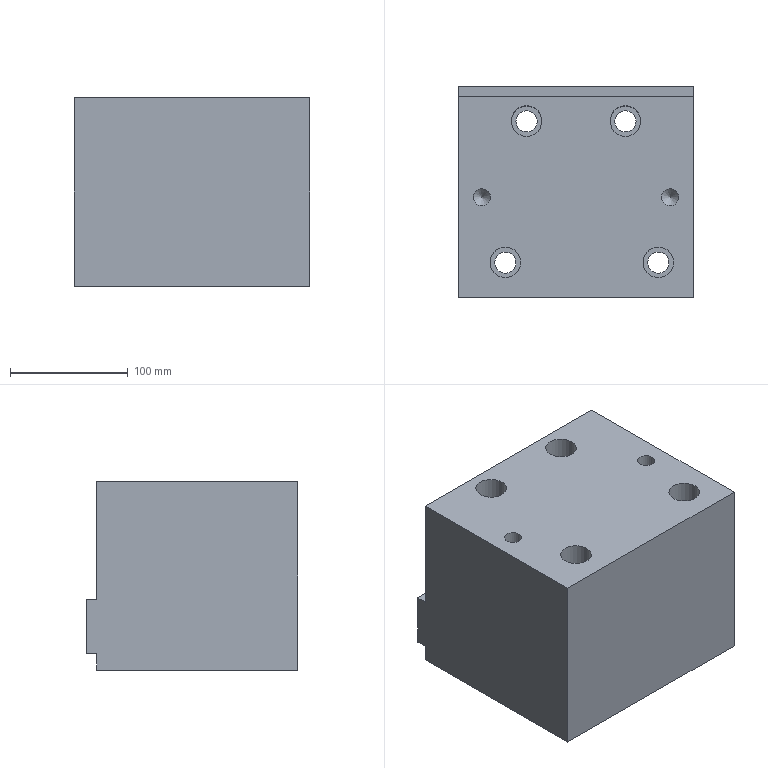Part | STEP file | lll_id4218_x_t | 1 solid | 34 faces | box 200 x 180 x 160 mm | volume 5239112 mm3 | plane 14 | cylinder 14 | cone 6 | commonest cylinder face diameters 8.506 x4 18.009 x4 26.008 x4 14.506 x2
STEP:
#1=CARTESIAN_POINT('',(1841.005,-387.377,-55.));
#2=VERTEX_POINT('',#1);
#3=CARTESIAN_POINT('',(1832.,-387.377,-55.));
#4=DIRECTION('',(0.,0.,1.));
#5=DIRECTION('',(1.,0.,0.));
#6=AXIS2_PLACEMENT_3D('',#3,#4,#5);
#7=CIRCLE('',#6,9.005);
#8=EDGE_CURVE('',#2,#2,#7,.T.);
#9=ORIENTED_EDGE('',*,*,#8,.F.);
#10=EDGE_LOOP('',(#9));
#11=FACE_BOUND('',#10,.T.);
#12=CARTESIAN_POINT('',(1845.004,-387.377,-55.));
#13=VERTEX_POINT('',#12);
#14=CARTESIAN_POINT('',(1832.,-387.377,-55.));
#15=DIRECTION('',(0.,0.,1.));
#16=DIRECTION('',(1.,0.,0.));
#17=AXIS2_PLACEMENT_3D('',#14,#15,#16);
#18=CIRCLE('',#17,13.004);
#19=EDGE_CURVE('',#13,#13,#18,.T.);
#20=ORIENTED_EDGE('',*,*,#19,.T.);
#21=EDGE_LOOP('',(#20));
#22=FACE_BOUND('',#21,.T.);
#23=CARTESIAN_POINT('',(1832.,-387.377,-55.));
#24=DIRECTION('',(0.,0.,-1.));
#25=DIRECTION('',(-1.,0.,0.));
#26=AXIS2_PLACEMENT_3D('',#23,#24,#25);
#27=PLANE('',#26);
#28=ADVANCED_FACE('',(#11,#22),#27,.F.);
#29=ORIENTED_EDGE('',*,*,#8,.T.);
#30=EDGE_LOOP('',(#29));
#31=FACE_BOUND('',#30,.T.);
#32=CARTESIAN_POINT('',(1841.005,-387.377,-95.));
#33=VERTEX_POINT('',#32);
#34=CARTESIAN_POINT('',(1832.,-387.377,-95.));
#35=DIRECTION('',(0.,0.,1.));
#36=DIRECTION('',(1.,0.,0.));
#37=AXIS2_PLACEMENT_3D('',#34,#35,#36);
#38=CIRCLE('',#37,9.005);
#39=EDGE_CURVE('',#33,#33,#38,.T.);
#40=ORIENTED_EDGE('',*,*,#39,.F.);
#41=EDGE_LOOP('',(#40));
#42=FACE_BOUND('',#41,.T.);
#43=CARTESIAN_POINT('',(1832.,-387.377,67.));
#44=DIRECTION('',(0.,0.,-1.));
#45=DIRECTION('',(1.,0.,0.));
#46=AXIS2_PLACEMENT_3D('',#43,#44,#45);
#47=CYLINDRICAL_SURFACE('',#46,9.005);
#48=ADVANCED_FACE('',(#31,#42),#47,.F.);
#49=ORIENTED_EDGE('',*,*,#19,.F.);
#50=EDGE_LOOP('',(#49));
#51=FACE_BOUND('',#50,.T.);
#52=CARTESIAN_POINT('',(1845.004,-387.377,65.));
#53=VERTEX_POINT('',#52);
#54=CARTESIAN_POINT('',(1832.,-387.377,65.));
#55=DIRECTION('',(0.,0.,1.));
#56=DIRECTION('',(1.,0.,0.));
#57=AXIS2_PLACEMENT_3D('',#54,#55,#56);
#58=CIRCLE('',#57,13.004);
#59=EDGE_CURVE('',#53,#53,#58,.T.);
#60=ORIENTED_EDGE('',*,*,#59,.T.);
#61=EDGE_LOOP('',(#60));
#62=FACE_BOUND('',#61,.T.);
#63=CARTESIAN_POINT('',(1832.,-387.377,65.));
#64=DIRECTION('',(0.,0.,-1.));
#65=DIRECTION('',(1.,0.,0.));
#66=AXIS2_PLACEMENT_3D('',#63,#64,#65);
#67=CYLINDRICAL_SURFACE('',#66,13.004);
#68=ADVANCED_FACE('',(#51,#62),#67,.F.);
#69=CARTESIAN_POINT('',(1715.,-401.383,40.));
#70=VERTEX_POINT('',#69);
#71=VERTEX_LOOP('',#70);
#72=FACE_BOUND('',#71,.T.);
#73=CARTESIAN_POINT('',(1715.,-397.13,35.747));
#74=VERTEX_POINT('',#73);
#75=CARTESIAN_POINT('',(1715.,-397.13,40.));
#76=DIRECTION('',(0.,1.,0.));
#77=DIRECTION('',(0.,0.,-1.));
#78=AXIS2_PLACEMENT_3D('',#75,#76,#77);
#79=CIRCLE('',#78,4.253);
#80=EDGE_CURVE('',#74,#74,#79,.T.);
#81=ORIENTED_EDGE('',*,*,#80,.T.);
#82=EDGE_LOOP('',(#81));
#83=FACE_BOUND('',#82,.T.);
#84=CARTESIAN_POINT('',(1715.,-397.13,40.));
#85=DIRECTION('',(0.,1.,0.));
#86=DIRECTION('',(0.,0.,1.));
#87=AXIS2_PLACEMENT_3D('',#84,#85,#86);
#88=CONICAL_SURFACE('',#87,4.253,45.);
#89=ADVANCED_FACE('',(#72,#83),#88,.F.);
#90=CARTESIAN_POINT('',(1865.,-401.383,40.));
#91=VERTEX_POINT('',#90);
#92=VERTEX_LOOP('',#91);
#93=FACE_BOUND('',#92,.T.);
#94=CARTESIAN_POINT('',(1865.,-397.13,35.747));
#95=VERTEX_POINT('',#94);
#96=CARTESIAN_POINT('',(1865.,-397.13,40.));
#97=DIRECTION('',(0.,1.,0.));
#98=DIRECTION('',(0.,0.,-1.));
#99=AXIS2_PLACEMENT_3D('',#96,#97,#98);
#100=CIRCLE('',#99,4.253);
#101=EDGE_CURVE('',#95,#95,#100,.T.);
#102=ORIENTED_EDGE('',*,*,#101,.T.);
#103=EDGE_LOOP('',(#102));
#104=FACE_BOUND('',#103,.T.);
#105=CARTESIAN_POINT('',(1865.,-397.13,40.));
#106=DIRECTION('',(0.,1.,0.));
#107=DIRECTION('',(0.,0.,1.));
#108=AXIS2_PLACEMENT_3D('',#105,#106,#107);
#109=CONICAL_SURFACE('',#108,4.253,45.);
#110=ADVANCED_FACE('',(#93,#104),#109,.F.);
#111=CARTESIAN_POINT('',(1715.,-401.383,-10.));
#112=VERTEX_POINT('',#111);
#113=VERTEX_LOOP('',#112);
#114=FACE_BOUND('',#113,.T.);
#115=CARTESIAN_POINT('',(1715.,-397.13,-14.253));
#116=VERTEX_POINT('',#115);
#117=CARTESIAN_POINT('',(1715.,-397.13,-10.));
#118=DIRECTION('',(0.,1.,0.));
#119=DIRECTION('',(0.,0.,-1.));
#120=AXIS2_PLACEMENT_3D('',#117,#118,#119);
#121=CIRCLE('',#120,4.253);
#122=EDGE_CURVE('',#116,#116,#121,.T.);
#123=ORIENTED_EDGE('',*,*,#122,.T.);
#124=EDGE_LOOP('',(#123));
#125=FACE_BOUND('',#124,.T.);
#126=CARTESIAN_POINT('',(1715.,-397.13,-10.));
#127=DIRECTION('',(0.,1.,0.));
#128=DIRECTION('',(0.,0.,1.));
#129=AXIS2_PLACEMENT_3D('',#126,#127,#128);
#130=CONICAL_SURFACE('',#129,4.253,45.);
#131=ADVANCED_FACE('',(#114,#125),#130,.F.);
#132=CARTESIAN_POINT('',(1865.,-401.383,-10.));
#133=VERTEX_POINT('',#132);
#134=VERTEX_LOOP('',#133);
#135=FACE_BOUND('',#134,.T.);
#136=CARTESIAN_POINT('',(1865.,-397.13,-14.253));
#137=VERTEX_POINT('',#136);
#138=CARTESIAN_POINT('',(1865.,-397.13,-10.));
#139=DIRECTION('',(0.,1.,0.));
#140=DIRECTION('',(0.,0.,-1.));
#141=AXIS2_PLACEMENT_3D('',#138,#139,#140);
#142=CIRCLE('',#141,4.253);
#143=EDGE_CURVE('',#137,#137,#142,.T.);
#144=ORIENTED_EDGE('',*,*,#143,.T.);
#145=EDGE_LOOP('',(#144));
#146=FACE_BOUND('',#145,.T.);
#147=CARTESIAN_POINT('',(1865.,-397.13,-10.));
#148=DIRECTION('',(0.,1.,0.));
#149=DIRECTION('',(0.,0.,1.));
#150=AXIS2_PLACEMENT_3D('',#147,#148,#149);
#151=CONICAL_SURFACE('',#150,4.253,45.);
#152=ADVANCED_FACE('',(#135,#146),#151,.F.);
#153=CARTESIAN_POINT('',(1710.,-451.877,21.994));
#154=VERTEX_POINT('',#153);
#155=VERTEX_LOOP('',#154);
#156=FACE_BOUND('',#155,.T.);
#157=CARTESIAN_POINT('',(1717.253,-451.877,29.247));
#158=VERTEX_POINT('',#157);
#159=CARTESIAN_POINT('',(1710.,-451.877,29.247));
#160=DIRECTION('',(0.,0.,1.));
#161=DIRECTION('',(1.,0.,0.));
#162=AXIS2_PLACEMENT_3D('',#159,#160,#161);
#163=CIRCLE('',#162,7.253);
#164=EDGE_CURVE('',#158,#158,#163,.T.);
#165=ORIENTED_EDGE('',*,*,#164,.T.);
#166=EDGE_LOOP('',(#165));
#167=FACE_BOUND('',#166,.T.);
#168=CARTESIAN_POINT('',(1710.,-451.877,29.247));
#169=DIRECTION('',(0.,0.,1.));
#170=DIRECTION('',(-1.,0.,0.));
#171=AXIS2_PLACEMENT_3D('',#168,#169,#170);
#172=CONICAL_SURFACE('',#171,7.253,45.);
#173=ADVANCED_FACE('',(#156,#167),#172,.F.);
#174=ORIENTED_EDGE('',*,*,#80,.F.);
#175=EDGE_LOOP('',(#174));
#176=FACE_BOUND('',#175,.T.);
#177=CARTESIAN_POINT('',(1710.747,-366.377,40.));
#178=VERTEX_POINT('',#177);
#179=CARTESIAN_POINT('',(1715.,-366.377,40.));
#180=DIRECTION('',(0.,1.,0.));
#181=DIRECTION('',(-1.,0.,0.));
#182=AXIS2_PLACEMENT_3D('',#179,#180,#181);
#183=CIRCLE('',#182,4.253);
#184=EDGE_CURVE('',#178,#178,#183,.T.);
#185=ORIENTED_EDGE('',*,*,#184,.T.);
#186=EDGE_LOOP('',(#185));
#187=FACE_BOUND('',#186,.T.);
#188=CARTESIAN_POINT('',(1715.,-366.377,40.));
#189=DIRECTION('',(0.,-1.,0.));
#190=DIRECTION('',(-1.,0.,0.));
#191=AXIS2_PLACEMENT_3D('',#188,#189,#190);
#192=CYLINDRICAL_SURFACE('',#191,4.253);
#193=ADVANCED_FACE('',(#176,#187),#192,.F.);
#194=ORIENTED_EDGE('',*,*,#101,.F.);
#195=EDGE_LOOP('',(#194));
#196=FACE_BOUND('',#195,.T.);
#197=CARTESIAN_POINT('',(1860.747,-366.377,40.));
#198=VERTEX_POINT('',#197);
#199=CARTESIAN_POINT('',(1865.,-366.377,40.));
#200=DIRECTION('',(0.,1.,0.));
#201=DIRECTION('',(-1.,0.,0.));
#202=AXIS2_PLACEMENT_3D('',#199,#200,#201);
#203=CIRCLE('',#202,4.253);
#204=EDGE_CURVE('',#198,#198,#203,.T.);
#205=ORIENTED_EDGE('',*,*,#204,.T.);
#206=EDGE_LOOP('',(#205));
#207=FACE_BOUND('',#206,.T.);
#208=CARTESIAN_POINT('',(1865.,-366.377,40.));
#209=DIRECTION('',(0.,-1.,0.));
#210=DIRECTION('',(-1.,0.,0.));
#211=AXIS2_PLACEMENT_3D('',#208,#209,#210);
#212=CYLINDRICAL_SURFACE('',#211,4.253);
#213=ADVANCED_FACE('',(#196,#207),#212,.F.);
#214=ORIENTED_EDGE('',*,*,#122,.F.);
#215=EDGE_LOOP('',(#214));
#216=FACE_BOUND('',#215,.T.);
#217=CARTESIAN_POINT('',(1710.747,-366.377,-10.));
#218=VERTEX_POINT('',#217);
#219=CARTESIAN_POINT('',(1715.,-366.377,-10.));
#220=DIRECTION('',(0.,1.,0.));
#221=DIRECTION('',(-1.,0.,0.));
#222=AXIS2_PLACEMENT_3D('',#219,#220,#221);
#223=CIRCLE('',#222,4.253);
#224=EDGE_CURVE('',#218,#218,#223,.T.);
#225=ORIENTED_EDGE('',*,*,#224,.T.);
#226=EDGE_LOOP('',(#225));
#227=FACE_BOUND('',#226,.T.);
#228=CARTESIAN_POINT('',(1715.,-366.377,-10.));
#229=DIRECTION('',(0.,-1.,0.));
#230=DIRECTION('',(-1.,0.,0.));
#231=AXIS2_PLACEMENT_3D('',#228,#229,#230);
#232=CYLINDRICAL_SURFACE('',#231,4.253);
#233=ADVANCED_FACE('',(#216,#227),#232,.F.);
#234=ORIENTED_EDGE('',*,*,#143,.F.);
#235=EDGE_LOOP('',(#234));
#236=FACE_BOUND('',#235,.T.);
#237=CARTESIAN_POINT('',(1860.747,-366.377,-10.));
#238=VERTEX_POINT('',#237);
#239=CARTESIAN_POINT('',(1865.,-366.377,-10.));
#240=DIRECTION('',(0.,1.,0.));
#241=DIRECTION('',(-1.,0.,0.));
#242=AXIS2_PLACEMENT_3D('',#239,#240,#241);
#243=CIRCLE('',#242,4.253);
#244=EDGE_CURVE('',#238,#238,#243,.T.);
#245=ORIENTED_EDGE('',*,*,#244,.T.);
#246=EDGE_LOOP('',(#245));
#247=FACE_BOUND('',#246,.T.);
#248=CARTESIAN_POINT('',(1865.,-366.377,-10.));
#249=DIRECTION('',(0.,-1.,0.));
#250=DIRECTION('',(-1.,0.,0.));
#251=AXIS2_PLACEMENT_3D('',#248,#249,#250);
#252=CYLINDRICAL_SURFACE('',#251,4.253);
#253=ADVANCED_FACE('',(#236,#247),#252,.F.);
#254=CARTESIAN_POINT('',(1738.995,-387.377,-55.));
#255=VERTEX_POINT('',#254);
#256=CARTESIAN_POINT('',(1748.,-387.377,-55.));
#257=DIRECTION('',(0.,0.,1.));
#258=DIRECTION('',(-1.,0.,0.));
#259=AXIS2_PLACEMENT_3D('',#256,#257,#258);
#260=CIRCLE('',#259,9.005);
#261=EDGE_CURVE('',#255,#255,#260,.T.);
#262=ORIENTED_EDGE('',*,*,#261,.F.);
#263=EDGE_LOOP('',(#262));
#264=FACE_BOUND('',#263,.T.);
#265=CARTESIAN_POINT('',(1734.996,-387.377,-55.));
#266=VERTEX_POINT('',#265);
#267=CARTESIAN_POINT('',(1748.,-387.377,-55.));
#268=DIRECTION('',(0.,0.,1.));
#269=DIRECTION('',(-1.,0.,0.));
#270=AXIS2_PLACEMENT_3D('',#267,#268,#269);
#271=CIRCLE('',#270,13.004);
#272=EDGE_CURVE('',#266,#266,#271,.T.);
#273=ORIENTED_EDGE('',*,*,#272,.T.);
#274=EDGE_LOOP('',(#273));
#275=FACE_BOUND('',#274,.T.);
#276=CARTESIAN_POINT('',(1748.,-387.377,-55.));
#277=DIRECTION('',(0.,0.,-1.));
#278=DIRECTION('',(1.,0.,0.));
#279=AXIS2_PLACEMENT_3D('',#276,#277,#278);
#280=PLANE('',#279);
#281=ADVANCED_FACE('',(#264,#275),#280,.F.);
#282=CARTESIAN_POINT('',(1690.,-366.377,-35.));
#283=VERTEX_POINT('',#282);
#284=CARTESIAN_POINT('',(1890.,-366.377,-35.));
#285=VERTEX_POINT('',#284);
#286=CARTESIAN_POINT('',(1142.435,-366.377,-35.));
#287=DIRECTION('',(1.,0.,0.));
#288=VECTOR('',#287,1.);
#289=LINE('',#286,#288);
#290=EDGE_CURVE('',#283,#285,#289,.T.);
#291=ORIENTED_EDGE('',*,*,#290,.T.);
#292=CARTESIAN_POINT('',(1890.,-357.377,-35.));
#293=VERTEX_POINT('',#292);
#294=CARTESIAN_POINT('',(1890.,-26.33,-35.));
#295=DIRECTION('',(0.,-1.,0.));
#296=VECTOR('',#295,1.);
#297=LINE('',#294,#296);
#298=EDGE_CURVE('',#293,#285,#297,.T.);
#299=ORIENTED_EDGE('',*,*,#298,.F.);
#300=CARTESIAN_POINT('',(1690.,-357.377,-35.));
#301=VERTEX_POINT('',#300);
#302=CARTESIAN_POINT('',(1142.435,-357.377,-35.));
#303=DIRECTION('',(-1.,0.,0.));
#304=VECTOR('',#303,1.);
#305=LINE('',#302,#304);
#306=EDGE_CURVE('',#293,#301,#305,.T.);
#307=ORIENTED_EDGE('',*,*,#306,.T.);
#308=CARTESIAN_POINT('',(1690.,-376.377,-35.));
#309=DIRECTION('',(0.,-1.,0.));
#310=VECTOR('',#309,1.);
#311=LINE('',#308,#310);
#312=EDGE_CURVE('',#301,#283,#311,.T.);
#313=ORIENTED_EDGE('',*,*,#312,.T.);
#314=EDGE_LOOP('',(#291,#299,#307,#313));
#315=FACE_OUTER_BOUND('',#314,.T.);
#316=CARTESIAN_POINT('',(1142.435,-26.33,-35.));
#317=DIRECTION('',(0.,0.,1.));
#318=DIRECTION('',(1.,0.,0.));
#319=AXIS2_PLACEMENT_3D('',#316,#317,#318);
#320=PLANE('',#319);
#321=ADVANCED_FACE('',(#315),#320,.T.);
#322=CARTESIAN_POINT('',(1720.995,-507.377,-55.));
#323=VERTEX_POINT('',#322);
#324=CARTESIAN_POINT('',(1730.,-507.377,-55.));
#325=DIRECTION('',(0.,0.,1.));
#326=DIRECTION('',(-1.,0.,0.));
#327=AXIS2_PLACEMENT_3D('',#324,#325,#326);
#328=CIRCLE('',#327,9.005);
#329=EDGE_CURVE('',#323,#323,#328,.T.);
#330=ORIENTED_EDGE('',*,*,#329,.F.);
#331=EDGE_LOOP('',(#330));
#332=FACE_BOUND('',#331,.T.);
#333=CARTESIAN_POINT('',(1716.996,-507.377,-55.));
#334=VERTEX_POINT('',#333);
#335=CARTESIAN_POINT('',(1730.,-507.377,-55.));
#336=DIRECTION('',(0.,0.,1.));
#337=DIRECTION('',(-1.,0.,0.));
#338=AXIS2_PLACEMENT_3D('',#335,#336,#337);
#339=CIRCLE('',#338,13.004);
#340=EDGE_CURVE('',#334,#334,#339,.T.);
#341=ORIENTED_EDGE('',*,*,#340,.T.);
#342=EDGE_LOOP('',(#341));
#343=FACE_BOUND('',#342,.T.);
#344=CARTESIAN_POINT('',(1730.,-507.377,-55.));
#345=DIRECTION('',(0.,0.,-1.));
#346=DIRECTION('',(1.,0.,0.));
#347=AXIS2_PLACEMENT_3D('',#344,#345,#346);
#348=PLANE('',#347);
#349=ADVANCED_FACE('',(#332,#343),#348,.F.);
#350=ORIENTED_EDGE('',*,*,#340,.F.);
#351=EDGE_LOOP('',(#350));
#352=FACE_BOUND('',#351,.T.);
#353=CARTESIAN_POINT('',(1716.996,-507.377,65.));
#354=VERTEX_POINT('',#353);
#355=CARTESIAN_POINT('',(1730.,-507.377,65.));
#356=DIRECTION('',(0.,0.,1.));
#357=DIRECTION('',(-1.,0.,0.));
#358=AXIS2_PLACEMENT_3D('',#355,#356,#357);
#359=CIRCLE('',#358,13.004);
#360=EDGE_CURVE('',#354,#354,#359,.T.);
#361=ORIENTED_EDGE('',*,*,#360,.T.);
#362=EDGE_LOOP('',(#361));
#363=FACE_BOUND('',#362,.T.);
#364=CARTESIAN_POINT('',(1730.,-507.377,65.));
#365=DIRECTION('',(0.,0.,-1.));
#366=DIRECTION('',(-1.,0.,0.));
#367=AXIS2_PLACEMENT_3D('',#364,#365,#366);
#368=CYLINDRICAL_SURFACE('',#367,13.004);
#369=ADVANCED_FACE('',(#352,#363),#368,.F.);
#370=ORIENTED_EDGE('',*,*,#272,.F.);
#371=EDGE_LOOP('',(#370));
#372=FACE_BOUND('',#371,.T.);
#373=CARTESIAN_POINT('',(1734.996,-387.377,65.));
#374=VERTEX_POINT('',#373);
#375=CARTESIAN_POINT('',(1748.,-387.377,65.));
#376=DIRECTION('',(0.,0.,1.));
#377=DIRECTION('',(-1.,0.,0.));
#378=AXIS2_PLACEMENT_3D('',#375,#376,#377);
#379=CIRCLE('',#378,13.004);
#380=EDGE_CURVE('',#374,#374,#379,.T.);
#381=ORIENTED_EDGE('',*,*,#380,.T.);
#382=EDGE_LOOP('',(#381));
#383=FACE_BOUND('',#382,.T.);
#384=CARTESIAN_POINT('',(1748.,-387.377,65.));
#385=DIRECTION('',(0.,0.,-1.));
#386=DIRECTION('',(-1.,0.,0.));
#387=AXIS2_PLACEMENT_3D('',#384,#385,#386);
#388=CYLINDRICAL_SURFACE('',#387,13.004);
#389=ADVANCED_FACE('',(#372,#383),#388,.F.);
#390=CARTESIAN_POINT('',(1702.747,-451.877,65.));
#391=VERTEX_POINT('',#390);
#392=CARTESIAN_POINT('',(1710.,-451.877,65.));
#393=DIRECTION('',(0.,0.,-1.));
#394=DIRECTION('',(-1.,0.,0.));
#395=AXIS2_PLACEMENT_3D('',#392,#393,#394);
#396=CIRCLE('',#395,7.253);
#397=EDGE_CURVE('',#391,#391,#396,.T.);
#398=ORIENTED_EDGE('',*,*,#397,.F.);
#399=EDGE_LOOP('',(#398));
#400=FACE_BOUND('',#399,.T.);
#401=ORIENTED_EDGE('',*,*,#164,.F.);
#402=EDGE_LOOP('',(#401));
#403=FACE_BOUND('',#402,.T.);
#404=CARTESIAN_POINT('',(1710.,-451.877,67.));
#405=DIRECTION('',(0.,0.,-1.));
#406=DIRECTION('',(-1.,0.,0.));
#407=AXIS2_PLACEMENT_3D('',#404,#405,#406);
#408=CYLINDRICAL_SURFACE('',#407,7.253);
#409=ADVANCED_FACE('',(#400,#403),#408,.F.);
#410=ORIENTED_EDGE('',*,*,#244,.F.);
#411=EDGE_LOOP('',(#410));
#412=FACE_BOUND('',#411,.T.);
#413=ORIENTED_EDGE('',*,*,#224,.F.);
#414=EDGE_LOOP('',(#413));
#415=FACE_BOUND('',#414,.T.);
#416=ORIENTED_EDGE('',*,*,#204,.F.);
#417=EDGE_LOOP('',(#416));
#418=FACE_BOUND('',#417,.T.);
#419=ORIENTED_EDGE('',*,*,#184,.F.);
#420=EDGE_LOOP('',(#419));
#421=FACE_BOUND('',#420,.T.);
#422=CARTESIAN_POINT('',(1890.,-366.377,65.));
#423=VERTEX_POINT('',#422);
#424=CARTESIAN_POINT('',(1690.,-366.377,65.));
#425=VERTEX_POINT('',#424);
#426=CARTESIAN_POINT('',(1665.,-366.377,65.));
#427=DIRECTION('',(-1.,0.,0.));
#428=VECTOR('',#427,1.);
#429=LINE('',#426,#428);
#430=EDGE_CURVE('',#423,#425,#429,.T.);
#431=ORIENTED_EDGE('',*,*,#430,.F.);
#432=CARTESIAN_POINT('',(1890.,-366.377,130.851));
#433=DIRECTION('',(0.,0.,-1.));
#434=VECTOR('',#433,1.);
#435=LINE('',#432,#434);
#436=EDGE_CURVE('',#423,#285,#435,.T.);
#437=ORIENTED_EDGE('',*,*,#436,.T.);
#438=ORIENTED_EDGE('',*,*,#290,.F.);
#439=CARTESIAN_POINT('',(1690.,-366.377,130.851));
#440=DIRECTION('',(0.,0.,-1.));
#441=VECTOR('',#440,1.);
#442=LINE('',#439,#441);
#443=EDGE_CURVE('',#425,#283,#442,.T.);
#444=ORIENTED_EDGE('',*,*,#443,.F.);
#445=EDGE_LOOP('',(#431,#437,#438,#444));
#446=FACE_BOUND('',#445,.T.);
#447=CARTESIAN_POINT('',(1695.,-366.377,130.851));
#448=DIRECTION('',(0.,-1.,0.));
#449=DIRECTION('',(0.,0.,-1.));
#450=AXIS2_PLACEMENT_3D('',#447,#448,#449);
#451=PLANE('',#450);
#452=ADVANCED_FACE('',(#412,#415,#418,#421,#446),#451,.F.);
#453=ORIENTED_EDGE('',*,*,#261,.T.);
#454=EDGE_LOOP('',(#453));
#455=FACE_BOUND('',#454,.T.);
#456=CARTESIAN_POINT('',(1757.005,-387.377,-95.));
#457=VERTEX_POINT('',#456);
#458=CARTESIAN_POINT('',(1748.,-387.377,-95.));
#459=DIRECTION('',(0.,0.,-1.));
#460=DIRECTION('',(1.,0.,0.));
#461=AXIS2_PLACEMENT_3D('',#458,#459,#460);
#462=CIRCLE('',#461,9.005);
#463=EDGE_CURVE('',#457,#457,#462,.T.);
#464=ORIENTED_EDGE('',*,*,#463,.T.);
#465=EDGE_LOOP('',(#464));
#466=FACE_BOUND('',#465,.T.);
#467=CARTESIAN_POINT('',(1748.,-387.377,67.));
#468=DIRECTION('',(0.,0.,-1.));
#469=DIRECTION('',(-1.,0.,0.));
#470=AXIS2_PLACEMENT_3D('',#467,#468,#469);
#471=CYLINDRICAL_SURFACE('',#470,9.005);
#472=ADVANCED_FACE('',(#455,#466),#471,.F.);
#473=CARTESIAN_POINT('',(1890.,-537.377,-95.));
#474=VERTEX_POINT('',#473);
#475=CARTESIAN_POINT('',(1890.,-537.377,65.));
#476=VERTEX_POINT('',#475);
#477=CARTESIAN_POINT('',(1890.,-537.377,-120.));
#478=DIRECTION('',(0.,0.,1.));
#479=VECTOR('',#478,1.);
#480=LINE('',#477,#479);
#481=EDGE_CURVE('',#474,#476,#480,.T.);
#482=ORIENTED_EDGE('',*,*,#481,.F.);
#483=CARTESIAN_POINT('',(1890.,-366.377,-95.));
#484=VERTEX_POINT('',#483);
#485=CARTESIAN_POINT('',(1890.,-416.877,-95.));
#486=DIRECTION('',(0.,-1.,0.));
#487=VECTOR('',#486,1.);
#488=LINE('',#485,#487);
#489=EDGE_CURVE('',#484,#474,#488,.T.);
#490=ORIENTED_EDGE('',*,*,#489,.F.);
#491=CARTESIAN_POINT('',(1890.,-366.377,-81.));
#492=VERTEX_POINT('',#491);
#493=CARTESIAN_POINT('',(1890.,-366.377,130.851));
#494=DIRECTION('',(0.,0.,1.));
#495=VECTOR('',#494,1.);
#496=LINE('',#493,#495);
#497=EDGE_CURVE('',#484,#492,#496,.T.);
#498=ORIENTED_EDGE('',*,*,#497,.T.);
#499=CARTESIAN_POINT('',(1890.,-357.377,-81.));
#500=VERTEX_POINT('',#499);
#501=CARTESIAN_POINT('',(1890.,-416.877,-81.));
#502=DIRECTION('',(0.,1.,0.));
#503=VECTOR('',#502,1.);
#504=LINE('',#501,#503);
#505=EDGE_CURVE('',#492,#500,#504,.T.);
#506=ORIENTED_EDGE('',*,*,#505,.T.);
#507=CARTESIAN_POINT('',(1890.,-357.377,-690.));
#508=DIRECTION('',(0.,0.,1.));
#509=VECTOR('',#508,1.);
#510=LINE('',#507,#509);
#511=EDGE_CURVE('',#500,#293,#510,.T.);
#512=ORIENTED_EDGE('',*,*,#511,.T.);
#513=ORIENTED_EDGE('',*,*,#298,.T.);
#514=ORIENTED_EDGE('',*,*,#436,.F.);
#515=CARTESIAN_POINT('',(1890.,-293.877,65.));
#516=DIRECTION('',(0.,1.,0.));
#517=VECTOR('',#516,1.);
#518=LINE('',#515,#517);
#519=EDGE_CURVE('',#476,#423,#518,.T.);
#520=ORIENTED_EDGE('',*,*,#519,.F.);
#521=EDGE_LOOP('',(#482,#490,#498,#506,#512,#513,#514,#520));
#522=FACE_OUTER_BOUND('',#521,.T.);
#523=CARTESIAN_POINT('',(1890.,-416.877,-35.));
#524=DIRECTION('',(-1.,0.,0.));
#525=DIRECTION('',(0.,0.,1.));
#526=AXIS2_PLACEMENT_3D('',#523,#524,#525);
#527=PLANE('',#526);
#528=ADVANCED_FACE('',(#522),#527,.F.);
#529=CARTESIAN_POINT('',(1690.,-357.377,-81.));
#530=VERTEX_POINT('',#529);
#531=CARTESIAN_POINT('',(-3186.249,-357.377,-81.));
#532=DIRECTION('',(1.,0.,0.));
#533=VECTOR('',#532,1.);
#534=LINE('',#531,#533);
#535=EDGE_CURVE('',#530,#500,#534,.T.);
#536=ORIENTED_EDGE('',*,*,#535,.F.);
#537=CARTESIAN_POINT('',(1690.,-357.377,-105.));
#538=DIRECTION('',(0.,0.,-1.));
#539=VECTOR('',#538,1.);
#540=LINE('',#537,#539);
#541=EDGE_CURVE('',#301,#530,#540,.T.);
#542=ORIENTED_EDGE('',*,*,#541,.F.);
#543=ORIENTED_EDGE('',*,*,#306,.F.);
#544=ORIENTED_EDGE('',*,*,#511,.F.);
#545=EDGE_LOOP('',(#536,#542,#543,#544));
#546=FACE_OUTER_BOUND('',#545,.T.);
#547=CARTESIAN_POINT('',(-3186.249,-357.377,-690.));
#548=DIRECTION('',(0.,1.,0.));
#549=DIRECTION('',(0.,0.,1.));
#550=AXIS2_PLACEMENT_3D('',#547,#548,#549);
#551=PLANE('',#550);
#552=ADVANCED_FACE('',(#546),#551,.T.);
#553=ORIENTED_EDGE('',*,*,#541,.T.);
#554=CARTESIAN_POINT('',(1690.,-366.377,-81.));
#555=VERTEX_POINT('',#554);
#556=CARTESIAN_POINT('',(1690.,-376.377,-81.));
#557=DIRECTION('',(0.,-1.,0.));
#558=VECTOR('',#557,1.);
#559=LINE('',#556,#558);
#560=EDGE_CURVE('',#530,#555,#559,.T.);
#561=ORIENTED_EDGE('',*,*,#560,.T.);
#562=CARTESIAN_POINT('',(1690.,-366.377,-95.));
#563=VERTEX_POINT('',#562);
#564=CARTESIAN_POINT('',(1690.,-366.377,130.851));
#565=DIRECTION('',(0.,0.,-1.));
#566=VECTOR('',#565,1.);
#567=LINE('',#564,#566);
#568=EDGE_CURVE('',#555,#563,#567,.T.);
#569=ORIENTED_EDGE('',*,*,#568,.T.);
#570=CARTESIAN_POINT('',(1690.,-537.377,-95.));
#571=VERTEX_POINT('',#570);
#572=CARTESIAN_POINT('',(1690.,-376.377,-95.));
#573=DIRECTION('',(0.,-1.,0.));
#574=VECTOR('',#573,1.);
#575=LINE('',#572,#574);
#576=EDGE_CURVE('',#563,#571,#575,.T.);
#577=ORIENTED_EDGE('',*,*,#576,.T.);
#578=CARTESIAN_POINT('',(1690.,-537.377,65.));
#579=VERTEX_POINT('',#578);
#580=CARTESIAN_POINT('',(1690.,-537.377,-105.));
#581=DIRECTION('',(0.,0.,1.));
#582=VECTOR('',#581,1.);
#583=LINE('',#580,#582);
#584=EDGE_CURVE('',#571,#579,#583,.T.);
#585=ORIENTED_EDGE('',*,*,#584,.T.);
#586=CARTESIAN_POINT('',(1690.,-293.877,65.));
#587=DIRECTION('',(0.,-1.,0.));
#588=VECTOR('',#587,1.);
#589=LINE('',#586,#588);
#590=EDGE_CURVE('',#425,#579,#589,.T.);
#591=ORIENTED_EDGE('',*,*,#590,.F.);
#592=ORIENTED_EDGE('',*,*,#443,.T.);
#593=ORIENTED_EDGE('',*,*,#312,.F.);
#594=EDGE_LOOP('',(#553,#561,#569,#577,#585,#591,#592,#593));
#595=FACE_OUTER_BOUND('',#594,.T.);
#596=CARTESIAN_POINT('',(1690.,-376.377,-105.));
#597=DIRECTION('',(1.,0.,0.));
#598=DIRECTION('',(0.,0.,1.));
#599=AXIS2_PLACEMENT_3D('',#596,#597,#598);
#600=PLANE('',#599);
#601=ADVANCED_FACE('',(#595),#600,.F.);
#602=ORIENTED_EDGE('',*,*,#584,.F.);
#603=CARTESIAN_POINT('',(1665.,-537.377,-95.));
#604=DIRECTION('',(1.,0.,0.));
#605=VECTOR('',#604,1.);
#606=LINE('',#603,#605);
#607=EDGE_CURVE('',#571,#474,#606,.T.);
#608=ORIENTED_EDGE('',*,*,#607,.T.);
#609=ORIENTED_EDGE('',*,*,#481,.T.);
#610=CARTESIAN_POINT('',(1665.,-537.377,65.));
#611=DIRECTION('',(1.,0.,0.));
#612=VECTOR('',#611,1.);
#613=LINE('',#610,#612);
#614=EDGE_CURVE('',#579,#476,#613,.T.);
#615=ORIENTED_EDGE('',*,*,#614,.F.);
#616=EDGE_LOOP('',(#602,#608,#609,#615));
#617=FACE_OUTER_BOUND('',#616,.T.);
#618=CARTESIAN_POINT('',(1665.,-537.377,-120.));
#619=DIRECTION('',(0.,-1.,0.));
#620=DIRECTION('',(0.,0.,-1.));
#621=AXIS2_PLACEMENT_3D('',#618,#619,#620);
#622=PLANE('',#621);
#623=ADVANCED_FACE('',(#617),#622,.T.);
#624=ORIENTED_EDGE('',*,*,#329,.T.);
#625=EDGE_LOOP('',(#624));
#626=FACE_BOUND('',#625,.T.);
#627=CARTESIAN_POINT('',(1739.005,-507.377,-95.));
#628=VERTEX_POINT('',#627);
#629=CARTESIAN_POINT('',(1730.,-507.377,-95.));
#630=DIRECTION('',(0.,0.,-1.));
#631=DIRECTION('',(1.,0.,0.));
#632=AXIS2_PLACEMENT_3D('',#629,#630,#631);
#633=CIRCLE('',#632,9.005);
#634=EDGE_CURVE('',#628,#628,#633,.T.);
#635=ORIENTED_EDGE('',*,*,#634,.T.);
#636=EDGE_LOOP('',(#635));
#637=FACE_BOUND('',#636,.T.);
#638=CARTESIAN_POINT('',(1730.,-507.377,67.));
#639=DIRECTION('',(0.,0.,-1.));
#640=DIRECTION('',(-1.,0.,0.));
#641=AXIS2_PLACEMENT_3D('',#638,#639,#640);
#642=CYLINDRICAL_SURFACE('',#641,9.005);
#643=ADVANCED_FACE('',(#626,#637),#642,.F.);
#644=ORIENTED_EDGE('',*,*,#590,.T.);
#645=ORIENTED_EDGE('',*,*,#614,.T.);
#646=ORIENTED_EDGE('',*,*,#519,.T.);
#647=ORIENTED_EDGE('',*,*,#430,.T.);
#648=EDGE_LOOP('',(#644,#645,#646,#647));
#649=FACE_BOUND('',#648,.T.);
#650=CARTESIAN_POINT('',(1873.004,-507.377,65.));
#651=VERTEX_POINT('',#650);
#652=CARTESIAN_POINT('',(1860.,-507.377,65.));
#653=DIRECTION('',(0.,0.,1.));
#654=DIRECTION('',(1.,0.,0.));
#655=AXIS2_PLACEMENT_3D('',#652,#653,#654);
#656=CIRCLE('',#655,13.004);
#657=EDGE_CURVE('',#651,#651,#656,.T.);
#658=ORIENTED_EDGE('',*,*,#657,.F.);
#659=EDGE_LOOP('',(#658));
#660=FACE_BOUND('',#659,.T.);
#661=ORIENTED_EDGE('',*,*,#59,.F.);
#662=EDGE_LOOP('',(#661));
#663=FACE_BOUND('',#662,.T.);
#664=CARTESIAN_POINT('',(1877.253,-451.877,65.));
#665=VERTEX_POINT('',#664);
#666=CARTESIAN_POINT('',(1870.,-451.877,65.));
#667=DIRECTION('',(0.,0.,1.));
#668=DIRECTION('',(1.,0.,0.));
#669=AXIS2_PLACEMENT_3D('',#666,#667,#668);
#670=CIRCLE('',#669,7.253);
#671=EDGE_CURVE('',#665,#665,#670,.T.);
#672=ORIENTED_EDGE('',*,*,#671,.F.);
#673=EDGE_LOOP('',(#672));
#674=FACE_BOUND('',#673,.T.);
#675=ORIENTED_EDGE('',*,*,#397,.T.);
#676=EDGE_LOOP('',(#675));
#677=FACE_BOUND('',#676,.T.);
#678=ORIENTED_EDGE('',*,*,#380,.F.);
#679=EDGE_LOOP('',(#678));
#680=FACE_BOUND('',#679,.T.);
#681=ORIENTED_EDGE('',*,*,#360,.F.);
#682=EDGE_LOOP('',(#681));
#683=FACE_BOUND('',#682,.T.);
#684=CARTESIAN_POINT('',(1665.,-293.877,65.));
#685=DIRECTION('',(0.,0.,1.));
#686=DIRECTION('',(-1.,0.,0.));
#687=AXIS2_PLACEMENT_3D('',#684,#685,#686);
#688=PLANE('',#687);
#689=ADVANCED_FACE('',(#649,#660,#663,#674,#677,#680,#683),#688,.T.);
#690=CARTESIAN_POINT('',(1869.005,-507.377,-55.));
#691=VERTEX_POINT('',#690);
#692=CARTESIAN_POINT('',(1860.,-507.377,-55.));
#693=DIRECTION('',(0.,0.,1.));
#694=DIRECTION('',(1.,0.,0.));
#695=AXIS2_PLACEMENT_3D('',#692,#693,#694);
#696=CIRCLE('',#695,9.005);
#697=EDGE_CURVE('',#691,#691,#696,.T.);
#698=ORIENTED_EDGE('',*,*,#697,.F.);
#699=EDGE_LOOP('',(#698));
#700=FACE_BOUND('',#699,.T.);
#701=CARTESIAN_POINT('',(1873.004,-507.377,-55.));
#702=VERTEX_POINT('',#701);
#703=CARTESIAN_POINT('',(1860.,-507.377,-55.));
#704=DIRECTION('',(0.,0.,1.));
#705=DIRECTION('',(1.,0.,0.));
#706=AXIS2_PLACEMENT_3D('',#703,#704,#705);
#707=CIRCLE('',#706,13.004);
#708=EDGE_CURVE('',#702,#702,#707,.T.);
#709=ORIENTED_EDGE('',*,*,#708,.T.);
#710=EDGE_LOOP('',(#709));
#711=FACE_BOUND('',#710,.T.);
#712=CARTESIAN_POINT('',(1860.,-507.377,-55.));
#713=DIRECTION('',(0.,0.,-1.));
#714=DIRECTION('',(-1.,0.,0.));
#715=AXIS2_PLACEMENT_3D('',#712,#713,#714);
#716=PLANE('',#715);
#717=ADVANCED_FACE('',(#700,#711),#716,.F.);
#718=ORIENTED_EDGE('',*,*,#697,.T.);
#719=EDGE_LOOP('',(#718));
#720=FACE_BOUND('',#719,.T.);
#721=CARTESIAN_POINT('',(1869.005,-507.377,-95.));
#722=VERTEX_POINT('',#721);
#723=CARTESIAN_POINT('',(1860.,-507.377,-95.));
#724=DIRECTION('',(0.,0.,1.));
#725=DIRECTION('',(1.,0.,0.));
#726=AXIS2_PLACEMENT_3D('',#723,#724,#725);
#727=CIRCLE('',#726,9.005);
#728=EDGE_CURVE('',#722,#722,#727,.T.);
#729=ORIENTED_EDGE('',*,*,#728,.F.);
#730=EDGE_LOOP('',(#729));
#731=FACE_BOUND('',#730,.T.);
#732=CARTESIAN_POINT('',(1860.,-507.377,67.));
#733=DIRECTION('',(0.,0.,-1.));
#734=DIRECTION('',(1.,0.,0.));
#735=AXIS2_PLACEMENT_3D('',#732,#733,#734);
#736=CYLINDRICAL_SURFACE('',#735,9.005);
#737=ADVANCED_FACE('',(#720,#731),#736,.F.);
#738=ORIENTED_EDGE('',*,*,#708,.F.);
#739=EDGE_LOOP('',(#738));
#740=FACE_BOUND('',#739,.T.);
#741=ORIENTED_EDGE('',*,*,#657,.T.);
#742=EDGE_LOOP('',(#741));
#743=FACE_BOUND('',#742,.T.);
#744=CARTESIAN_POINT('',(1860.,-507.377,65.));
#745=DIRECTION('',(0.,0.,-1.));
#746=DIRECTION('',(1.,0.,0.));
#747=AXIS2_PLACEMENT_3D('',#744,#745,#746);
#748=CYLINDRICAL_SURFACE('',#747,13.004);
#749=ADVANCED_FACE('',(#740,#743),#748,.F.);
#750=CARTESIAN_POINT('',(1870.,-451.877,21.994));
#751=VERTEX_POINT('',#750);
#752=VERTEX_LOOP('',#751);
#753=FACE_BOUND('',#752,.T.);
#754=CARTESIAN_POINT('',(1862.747,-451.877,29.247));
#755=VERTEX_POINT('',#754);
#756=CARTESIAN_POINT('',(1870.,-451.877,29.247));
#757=DIRECTION('',(0.,0.,1.));
#758=DIRECTION('',(-1.,0.,0.));
#759=AXIS2_PLACEMENT_3D('',#756,#757,#758);
#760=CIRCLE('',#759,7.253);
#761=EDGE_CURVE('',#755,#755,#760,.T.);
#762=ORIENTED_EDGE('',*,*,#761,.T.);
#763=EDGE_LOOP('',(#762));
#764=FACE_BOUND('',#763,.T.);
#765=CARTESIAN_POINT('',(1870.,-451.877,29.247));
#766=DIRECTION('',(0.,0.,1.));
#767=DIRECTION('',(1.,0.,0.));
#768=AXIS2_PLACEMENT_3D('',#765,#766,#767);
#769=CONICAL_SURFACE('',#768,7.253,45.);
#770=ADVANCED_FACE('',(#753,#764),#769,.F.);
#771=ORIENTED_EDGE('',*,*,#671,.T.);
#772=EDGE_LOOP('',(#771));
#773=FACE_BOUND('',#772,.T.);
#774=ORIENTED_EDGE('',*,*,#761,.F.);
#775=EDGE_LOOP('',(#774));
#776=FACE_BOUND('',#775,.T.);
#777=CARTESIAN_POINT('',(1870.,-451.877,67.));
#778=DIRECTION('',(0.,0.,-1.));
#779=DIRECTION('',(1.,0.,0.));
#780=AXIS2_PLACEMENT_3D('',#777,#778,#779);
#781=CYLINDRICAL_SURFACE('',#780,7.253);
#782=ADVANCED_FACE('',(#773,#776),#781,.F.);
#783=ORIENTED_EDGE('',*,*,#505,.F.);
#784=CARTESIAN_POINT('',(2067.435,-366.377,-81.));
#785=DIRECTION('',(-1.,0.,0.));
#786=VECTOR('',#785,1.);
#787=LINE('',#784,#786);
#788=EDGE_CURVE('',#492,#555,#787,.T.);
#789=ORIENTED_EDGE('',*,*,#788,.T.);
#790=ORIENTED_EDGE('',*,*,#560,.F.);
#791=ORIENTED_EDGE('',*,*,#535,.T.);
#792=EDGE_LOOP('',(#783,#789,#790,#791));
#793=FACE_OUTER_BOUND('',#792,.T.);
#794=CARTESIAN_POINT('',(2067.435,0.000000688,-81.));
#795=DIRECTION('',(0.,0.,1.));
#796=DIRECTION('',(-1.,0.,0.));
#797=AXIS2_PLACEMENT_3D('',#794,#795,#796);
#798=PLANE('',#797);
#799=ADVANCED_FACE('',(#793),#798,.F.);
#800=ORIENTED_EDGE('',*,*,#568,.F.);
#801=ORIENTED_EDGE('',*,*,#788,.F.);
#802=ORIENTED_EDGE('',*,*,#497,.F.);
#803=CARTESIAN_POINT('',(1695.,-366.377,-95.));
#804=DIRECTION('',(1.,0.,0.));
#805=VECTOR('',#804,1.);
#806=LINE('',#803,#805);
#807=EDGE_CURVE('',#563,#484,#806,.T.);
#808=ORIENTED_EDGE('',*,*,#807,.F.);
#809=EDGE_LOOP('',(#800,#801,#802,#808));
#810=FACE_OUTER_BOUND('',#809,.T.);
#811=CARTESIAN_POINT('',(1695.,-366.377,130.851));
#812=DIRECTION('',(0.,-1.,0.));
#813=DIRECTION('',(0.,0.,-1.));
#814=AXIS2_PLACEMENT_3D('',#811,#812,#813);
#815=PLANE('',#814);
#816=ADVANCED_FACE('',(#810),#815,.F.);
#817=ORIENTED_EDGE('',*,*,#463,.F.);
#818=EDGE_LOOP('',(#817));
#819=FACE_BOUND('',#818,.T.);
#820=ORIENTED_EDGE('',*,*,#489,.T.);
#821=ORIENTED_EDGE('',*,*,#607,.F.);
#822=ORIENTED_EDGE('',*,*,#576,.F.);
#823=ORIENTED_EDGE('',*,*,#807,.T.);
#824=EDGE_LOOP('',(#820,#821,#822,#823));
#825=FACE_BOUND('',#824,.T.);
#826=ORIENTED_EDGE('',*,*,#634,.F.);
#827=EDGE_LOOP('',(#826));
#828=FACE_BOUND('',#827,.T.);
#829=ORIENTED_EDGE('',*,*,#39,.T.);
#830=EDGE_LOOP('',(#829));
#831=FACE_BOUND('',#830,.T.);
#832=ORIENTED_EDGE('',*,*,#728,.T.);
#833=EDGE_LOOP('',(#832));
#834=FACE_BOUND('',#833,.T.);
#835=CARTESIAN_POINT('',(2092.435,0.000000688,-95.));
#836=DIRECTION('',(0.,0.,1.));
#837=DIRECTION('',(1.,0.,0.));
#838=AXIS2_PLACEMENT_3D('',#835,#836,#837);
#839=PLANE('',#838);
#840=ADVANCED_FACE('',(#819,#825,#828,#831,#834),#839,.F.);
#841=CLOSED_SHELL('',(#28,#48,#68,#89,#110,#131,#152,#173,#193,#213,#233,#253,#281,#321,#349,#369,#389,#409,#452,#472,#528,#552,#601,#623,#643,#689,#717,#737,#749,#770,#782,#799,#816,#840));
#842=MANIFOLD_SOLID_BREP('',#841);
#843=(LENGTH_UNIT()NAMED_UNIT(*)SI_UNIT(.MILLI.,.METRE.));
#844=UNCERTAINTY_MEASURE_WITH_UNIT(LENGTH_MEASURE(0.00002),#843,'','');
#845=(NAMED_UNIT(*)PLANE_ANGLE_UNIT()SI_UNIT($,.RADIAN.));
#846=PLANE_ANGLE_MEASURE_WITH_UNIT(PLANE_ANGLE_MEASURE(0.01745),#845);
#847=DIMENSIONAL_EXPONENTS(0.,0.,0.,0.,0.,0.,0.);
#848=(CONVERSION_BASED_UNIT('DEGREE',#846)NAMED_UNIT(#847)PLANE_ANGLE_UNIT());
#849=(NAMED_UNIT(*)SI_UNIT($,.STERADIAN.)SOLID_ANGLE_UNIT());
#850=(GEOMETRIC_REPRESENTATION_CONTEXT(3)GLOBAL_UNCERTAINTY_ASSIGNED_CONTEXT((#844))GLOBAL_UNIT_ASSIGNED_CONTEXT((#843,#848,#849))REPRESENTATION_CONTEXT('',''));
#851=ADVANCED_BREP_SHAPE_REPRESENTATION('',(#842),#850);